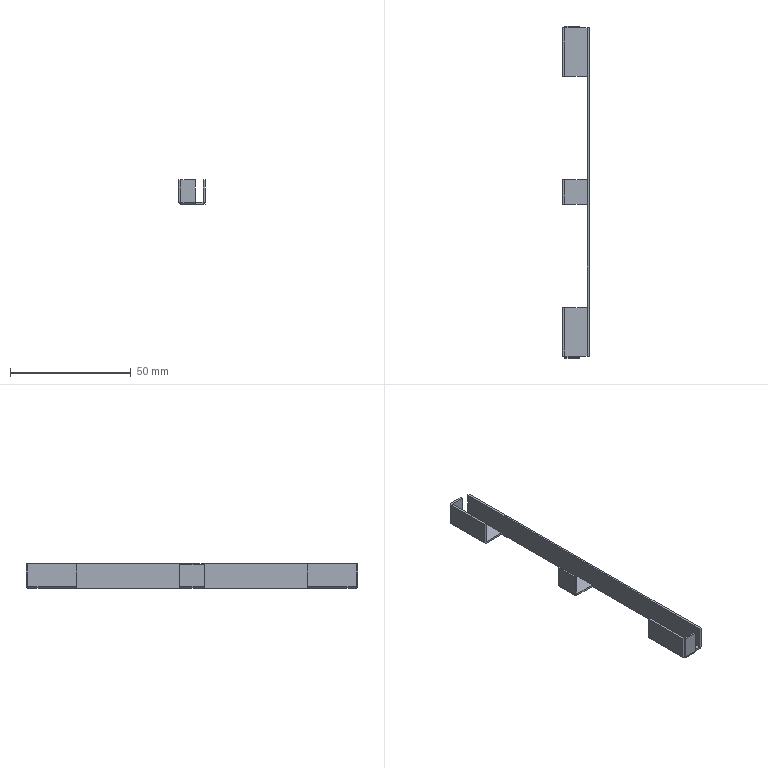Part | STEP file | RJWD-DY-0112_X2_4F20611F56685_2 | 1 solid | 50 faces | box 10.8 x 137.602 x 10 mm | volume 1934 mm3 | plane 42 | cylinder 8 | commonest cylinder face diameters 1.604 x8